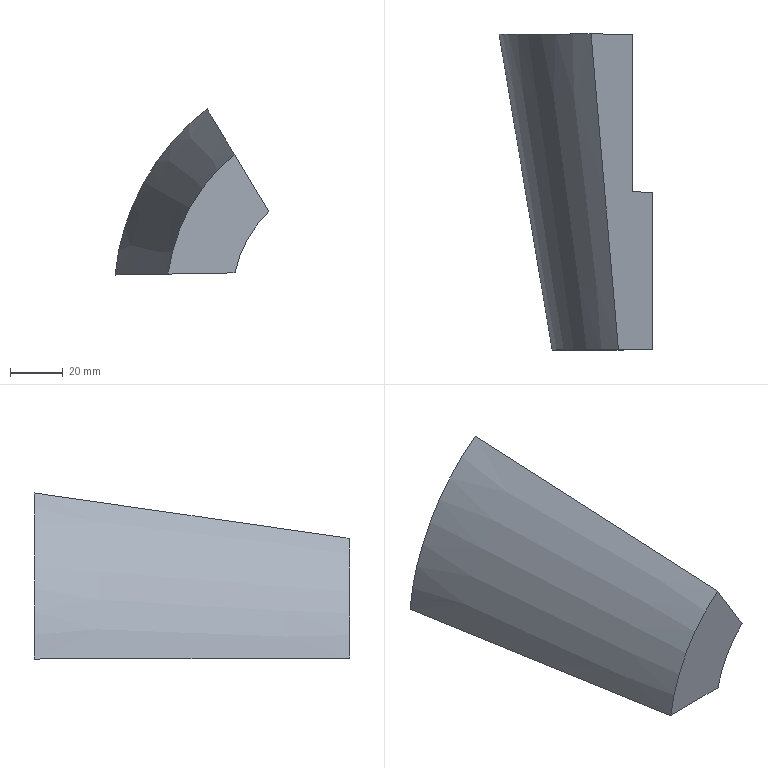Part | STEP file | 2026.6.15-Main Assembly图.sldasm-Part-59 | 1 solid | 8 faces | box 58.425 x 120 x 63.094 mm | volume 161225 mm3 | plane 5 | cylinder 2 | cone 1 | commonest cylinder face diameters 90 x1 120 x1
STEP:
#1=CARTESIAN_POINT('',(-798.384,648.541,3203.854));
#2=VERTEX_POINT('',#1);
#3=CARTESIAN_POINT('',(-785.52,648.541,3227.085));
#4=VERTEX_POINT('',#3);
#5=CARTESIAN_POINT('',(-754.337,648.541,3194.64));
#6=DIRECTION('',(0.,1.,0.));
#7=DIRECTION('',(0.5154,0.,-0.8569));
#8=AXIS2_PLACEMENT_3D('',#5,#6,#7);
#9=CIRCLE('',#8,45.);
#10=EDGE_CURVE('',#2,#4,#9,.T.);
#11=ORIENTED_EDGE('',*,*,#10,.F.);
#12=CARTESIAN_POINT('',(-798.384,708.541,3203.854));
#13=VERTEX_POINT('',#12);
#14=CARTESIAN_POINT('',(-798.384,648.541,3203.854));
#15=DIRECTION('',(0.,1.,0.));
#16=VECTOR('',#15,1000.);
#17=LINE('',#14,#16);
#18=EDGE_CURVE('',#2,#13,#17,.T.);
#19=ORIENTED_EDGE('',*,*,#18,.T.);
#20=CARTESIAN_POINT('',(-785.52,708.541,3227.085));
#21=VERTEX_POINT('',#20);
#22=CARTESIAN_POINT('',(-754.337,708.541,3194.64));
#23=DIRECTION('',(0.,-1.,0.));
#24=DIRECTION('',(0.5154,0.,-0.8569));
#25=AXIS2_PLACEMENT_3D('',#22,#23,#24);
#26=CIRCLE('',#25,45.);
#27=EDGE_CURVE('',#21,#13,#26,.T.);
#28=ORIENTED_EDGE('',*,*,#27,.F.);
#29=CARTESIAN_POINT('',(-785.52,648.541,3227.085));
#30=DIRECTION('',(0.,1.,0.));
#31=VECTOR('',#30,1000.);
#32=LINE('',#29,#31);
#33=EDGE_CURVE('',#4,#21,#32,.T.);
#34=ORIENTED_EDGE('',*,*,#33,.F.);
#35=EDGE_LOOP('',(#11,#19,#28,#34));
#36=FACE_OUTER_BOUND('',#35,.T.);
#37=CARTESIAN_POINT('',(-754.337,648.541,3194.64));
#38=DIRECTION('',(0.,1.,0.));
#39=DIRECTION('',(-0.5154,0.,0.8569));
#40=AXIS2_PLACEMENT_3D('',#37,#38,#39);
#41=CYLINDRICAL_SURFACE('',#40,45.);
#42=ADVANCED_FACE('',(#36),#41,.F.);
#43=CARTESIAN_POINT('',(-823.787,648.541,3203.4));
#44=VERTEX_POINT('',#43);
#45=CARTESIAN_POINT('',(-843.945,768.541,3203.04));
#46=VERTEX_POINT('',#45);
#47=CARTESIAN_POINT('',(-823.787,648.541,3203.4));
#48=CARTESIAN_POINT('',(-830.521,688.539,3203.28));
#49=CARTESIAN_POINT('',(-837.237,728.539,3203.159));
#50=CARTESIAN_POINT('',(-843.945,768.541,3203.04));
#51=B_SPLINE_CURVE_WITH_KNOTS('',3,(#47,#48,#49,#50),.UNSPECIFIED.,.F.,.F.,(4,4),(0.,0.1217),.UNSPECIFIED.);
#52=EDGE_CURVE('',#44,#46,#51,.T.);
#53=ORIENTED_EDGE('',*,*,#52,.F.);
#54=CARTESIAN_POINT('',(-798.615,648.541,3248.857));
#55=VERTEX_POINT('',#54);
#56=CARTESIAN_POINT('',(-754.337,648.541,3194.64));
#57=DIRECTION('',(0.,1.,0.));
#58=DIRECTION('',(0.5154,0.,-0.8569));
#59=AXIS2_PLACEMENT_3D('',#56,#57,#58);
#60=CIRCLE('',#59,70.);
#61=EDGE_CURVE('',#44,#55,#60,.T.);
#62=ORIENTED_EDGE('',*,*,#61,.T.);
#63=CARTESIAN_POINT('',(-809.006,768.541,3266.134));
#64=VERTEX_POINT('',#63);
#65=CARTESIAN_POINT('',(-809.006,768.541,3266.134));
#66=CARTESIAN_POINT('',(-805.548,728.539,3260.385));
#67=CARTESIAN_POINT('',(-802.086,688.539,3254.629));
#68=CARTESIAN_POINT('',(-798.615,648.541,3248.857));
#69=B_SPLINE_CURVE_WITH_KNOTS('',3,(#65,#66,#67,#68),.UNSPECIFIED.,.F.,.F.,(4,4),(0.,0.1217),.UNSPECIFIED.);
#70=EDGE_CURVE('',#64,#55,#69,.T.);
#71=ORIENTED_EDGE('',*,*,#70,.F.);
#72=CARTESIAN_POINT('',(-754.337,768.541,3194.64));
#73=DIRECTION('',(0.,1.,0.));
#74=DIRECTION('',(0.5154,0.,-0.8569));
#75=AXIS2_PLACEMENT_3D('',#72,#73,#74);
#76=CIRCLE('',#75,90.);
#77=EDGE_CURVE('',#46,#64,#76,.T.);
#78=ORIENTED_EDGE('',*,*,#77,.F.);
#79=EDGE_LOOP('',(#53,#62,#71,#78));
#80=FACE_OUTER_BOUND('',#79,.T.);
#81=CARTESIAN_POINT('',(-754.337,648.541,3194.64));
#82=DIRECTION('',(0.,1.,0.));
#83=DIRECTION('',(-0.5154,0.,0.8569));
#84=AXIS2_PLACEMENT_3D('',#81,#82,#83);
#85=CONICAL_SURFACE('',#84,70.,0.1651);
#86=ADVANCED_FACE('',(#80),#85,.T.);
#87=CARTESIAN_POINT('',(-813.668,768.541,3203.581));
#88=VERTEX_POINT('',#87);
#89=CARTESIAN_POINT('',(-760.289,768.541,3204.535));
#90=DIRECTION('',(0.9998,0.,0.01788));
#91=VECTOR('',#90,1000.);
#92=LINE('',#89,#91);
#93=EDGE_CURVE('',#46,#88,#92,.T.);
#94=ORIENTED_EDGE('',*,*,#93,.F.);
#95=ORIENTED_EDGE('',*,*,#77,.T.);
#96=CARTESIAN_POINT('',(-793.399,768.541,3240.184));
#97=VERTEX_POINT('',#96);
#98=CARTESIAN_POINT('',(-765.883,768.541,3194.434));
#99=DIRECTION('',(-0.5154,0.,0.8569));
#100=VECTOR('',#99,1000.);
#101=LINE('',#98,#100);
#102=EDGE_CURVE('',#97,#64,#101,.T.);
#103=ORIENTED_EDGE('',*,*,#102,.F.);
#104=CARTESIAN_POINT('',(-754.337,768.541,3194.64));
#105=DIRECTION('',(0.,1.,0.));
#106=DIRECTION('',(0.5154,0.,-0.8569));
#107=AXIS2_PLACEMENT_3D('',#104,#105,#106);
#108=CIRCLE('',#107,60.);
#109=EDGE_CURVE('',#88,#97,#108,.T.);
#110=ORIENTED_EDGE('',*,*,#109,.F.);
#111=EDGE_LOOP('',(#94,#95,#103,#110));
#112=FACE_OUTER_BOUND('',#111,.T.);
#113=CARTESIAN_POINT('',(-754.337,768.541,3194.64));
#114=DIRECTION('',(0.,1.,0.));
#115=DIRECTION('',(0.8569,0.,0.5154));
#116=AXIS2_PLACEMENT_3D('',#113,#114,#115);
#117=PLANE('',#116);
#118=ADVANCED_FACE('',(#112),#117,.T.);
#119=ORIENTED_EDGE('',*,*,#61,.F.);
#120=CARTESIAN_POINT('',(-760.289,648.541,3204.535));
#121=DIRECTION('',(0.9998,0.,0.01788));
#122=VECTOR('',#121,1000.);
#123=LINE('',#120,#122);
#124=EDGE_CURVE('',#44,#2,#123,.T.);
#125=ORIENTED_EDGE('',*,*,#124,.T.);
#126=ORIENTED_EDGE('',*,*,#10,.T.);
#127=CARTESIAN_POINT('',(-765.883,648.541,3194.434));
#128=DIRECTION('',(-0.5154,0.,0.8569));
#129=VECTOR('',#128,1000.);
#130=LINE('',#127,#129);
#131=EDGE_CURVE('',#4,#55,#130,.T.);
#132=ORIENTED_EDGE('',*,*,#131,.T.);
#133=EDGE_LOOP('',(#119,#125,#126,#132));
#134=FACE_OUTER_BOUND('',#133,.T.);
#135=CARTESIAN_POINT('',(-754.337,648.541,3194.64));
#136=DIRECTION('',(0.,1.,0.));
#137=DIRECTION('',(0.8569,0.,0.5154));
#138=AXIS2_PLACEMENT_3D('',#135,#136,#137);
#139=PLANE('',#138);
#140=ADVANCED_FACE('',(#134),#139,.F.);
#141=CARTESIAN_POINT('',(-813.668,708.541,3203.581));
#142=VERTEX_POINT('',#141);
#143=CARTESIAN_POINT('',(-793.399,708.541,3240.184));
#144=VERTEX_POINT('',#143);
#145=CARTESIAN_POINT('',(-754.337,708.541,3194.64));
#146=DIRECTION('',(0.,1.,0.));
#147=DIRECTION('',(0.5154,0.,-0.8569));
#148=AXIS2_PLACEMENT_3D('',#145,#146,#147);
#149=CIRCLE('',#148,60.);
#150=EDGE_CURVE('',#142,#144,#149,.T.);
#151=ORIENTED_EDGE('',*,*,#150,.F.);
#152=CARTESIAN_POINT('',(-813.668,708.541,3203.581));
#153=DIRECTION('',(0.,1.,0.));
#154=VECTOR('',#153,1000.);
#155=LINE('',#152,#154);
#156=EDGE_CURVE('',#142,#88,#155,.T.);
#157=ORIENTED_EDGE('',*,*,#156,.T.);
#158=ORIENTED_EDGE('',*,*,#109,.T.);
#159=CARTESIAN_POINT('',(-793.399,708.541,3240.184));
#160=DIRECTION('',(0.,1.,0.));
#161=VECTOR('',#160,1000.);
#162=LINE('',#159,#161);
#163=EDGE_CURVE('',#144,#97,#162,.T.);
#164=ORIENTED_EDGE('',*,*,#163,.F.);
#165=EDGE_LOOP('',(#151,#157,#158,#164));
#166=FACE_OUTER_BOUND('',#165,.T.);
#167=CARTESIAN_POINT('',(-754.337,708.541,3194.64));
#168=DIRECTION('',(0.,1.,0.));
#169=DIRECTION('',(-0.5154,0.,0.8569));
#170=AXIS2_PLACEMENT_3D('',#167,#168,#169);
#171=CYLINDRICAL_SURFACE('',#170,60.);
#172=ADVANCED_FACE('',(#166),#171,.F.);
#173=CARTESIAN_POINT('',(-754.516,708.541,3204.638));
#174=DIRECTION('',(0.9998,0.,0.01788));
#175=VECTOR('',#174,1000.);
#176=LINE('',#173,#175);
#177=EDGE_CURVE('',#142,#13,#176,.T.);
#178=ORIENTED_EDGE('',*,*,#177,.F.);
#179=ORIENTED_EDGE('',*,*,#150,.T.);
#180=CARTESIAN_POINT('',(-765.883,708.541,3194.434));
#181=DIRECTION('',(0.5154,0.,-0.8569));
#182=VECTOR('',#181,1000.);
#183=LINE('',#180,#182);
#184=EDGE_CURVE('',#144,#21,#183,.T.);
#185=ORIENTED_EDGE('',*,*,#184,.T.);
#186=ORIENTED_EDGE('',*,*,#27,.T.);
#187=EDGE_LOOP('',(#178,#179,#185,#186));
#188=FACE_OUTER_BOUND('',#187,.T.);
#189=CARTESIAN_POINT('',(-754.337,708.541,3194.64));
#190=DIRECTION('',(0.,1.,0.));
#191=DIRECTION('',(0.8569,0.,0.5154));
#192=AXIS2_PLACEMENT_3D('',#189,#190,#191);
#193=PLANE('',#192);
#194=ADVANCED_FACE('',(#188),#193,.T.);
#195=ORIENTED_EDGE('',*,*,#184,.F.);
#196=ORIENTED_EDGE('',*,*,#163,.T.);
#197=ORIENTED_EDGE('',*,*,#102,.T.);
#198=ORIENTED_EDGE('',*,*,#70,.T.);
#199=ORIENTED_EDGE('',*,*,#131,.F.);
#200=ORIENTED_EDGE('',*,*,#33,.T.);
#201=EDGE_LOOP('',(#195,#196,#197,#198,#199,#200));
#202=FACE_OUTER_BOUND('',#201,.T.);
#203=CARTESIAN_POINT('',(-765.883,648.541,3194.434));
#204=DIRECTION('',(-0.8569,0.,-0.5154));
#205=DIRECTION('',(0.5154,0.,-0.8569));
#206=AXIS2_PLACEMENT_3D('',#203,#204,#205);
#207=PLANE('',#206);
#208=ADVANCED_FACE('',(#202),#207,.F.);
#209=ORIENTED_EDGE('',*,*,#52,.T.);
#210=ORIENTED_EDGE('',*,*,#93,.T.);
#211=ORIENTED_EDGE('',*,*,#156,.F.);
#212=ORIENTED_EDGE('',*,*,#177,.T.);
#213=ORIENTED_EDGE('',*,*,#18,.F.);
#214=ORIENTED_EDGE('',*,*,#124,.F.);
#215=EDGE_LOOP('',(#209,#210,#211,#212,#213,#214));
#216=FACE_OUTER_BOUND('',#215,.T.);
#217=CARTESIAN_POINT('',(-760.289,648.541,3204.535));
#218=DIRECTION('',(-0.01788,0.,0.9998));
#219=DIRECTION('',(-0.9998,0.,-0.01788));
#220=AXIS2_PLACEMENT_3D('',#217,#218,#219);
#221=PLANE('',#220);
#222=ADVANCED_FACE('',(#216),#221,.F.);
#223=CLOSED_SHELL('',(#42,#86,#118,#140,#172,#194,#208,#222));
#224=MANIFOLD_SOLID_BREP('',#223);
#225=CARTESIAN_POINT('',(0.,0.,0.));
#226=DIRECTION('',(0.,0.,1.));
#227=DIRECTION('',(1.,0.,0.));
#228=AXIS2_PLACEMENT_3D('',#225,#226,#227);
#229=(LENGTH_UNIT()NAMED_UNIT(*)SI_UNIT(.MILLI.,.METRE.));
#230=UNCERTAINTY_MEASURE_WITH_UNIT(LENGTH_MEASURE(0.00001),#229,'','');
#231=(NAMED_UNIT(*)PLANE_ANGLE_UNIT()SI_UNIT($,.RADIAN.));
#232=(NAMED_UNIT(*)SI_UNIT($,.STERADIAN.)SOLID_ANGLE_UNIT());
#233=(GEOMETRIC_REPRESENTATION_CONTEXT(3)GLOBAL_UNCERTAINTY_ASSIGNED_CONTEXT((#230))GLOBAL_UNIT_ASSIGNED_CONTEXT((#229,#231,#232))REPRESENTATION_CONTEXT('',''));
#234=ADVANCED_BREP_SHAPE_REPRESENTATION('',(#224,#228),#233);